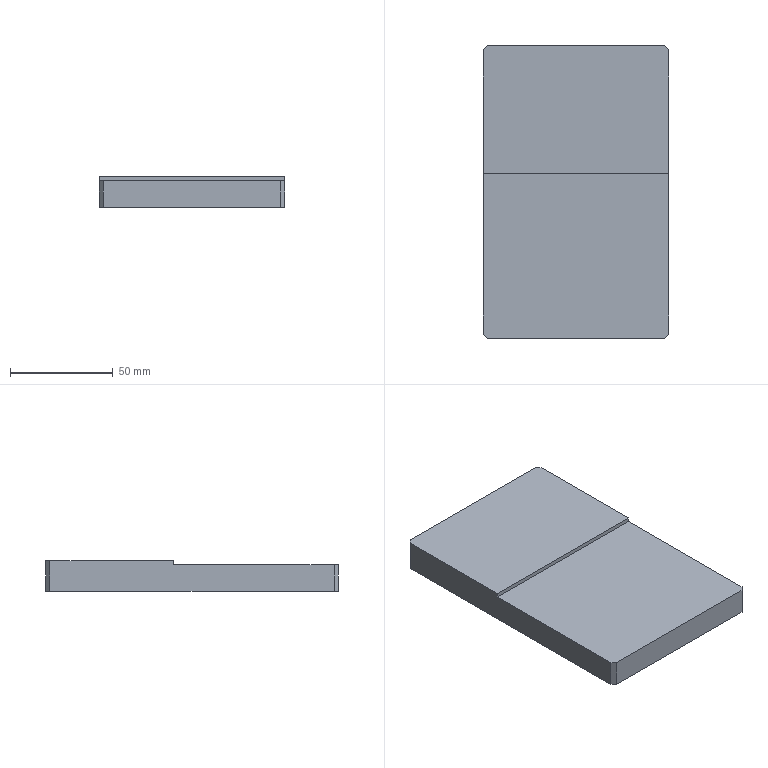Part | STEP file | 001-005-Shaft threading fixture adapter plate | 1 solid | 12 faces | box 90 x 142 x 15 mm | volume 177188 mm3 | plane 12
STEP:
#1=CARTESIAN_POINT('',(0.,0.,0.));
#2=DIRECTION('',(0.,0.,1.));
#3=DIRECTION('',(1.,0.,0.));
#4=AXIS2_PLACEMENT_3D('',#1,#2,#3);
#5=CARTESIAN_POINT('',(45.,9.,15.));
#6=VERTEX_POINT('',#5);
#7=CARTESIAN_POINT('',(45.,9.,13.));
#8=VERTEX_POINT('',#7);
#9=CARTESIAN_POINT('',(45.,9.,15.));
#10=DIRECTION('',(0.,0.,-1.));
#11=VECTOR('',#10,1.);
#12=LINE('',#9,#11);
#13=CARTESIAN_POINT('',(45.,-71.,15.));
#14=DIRECTION('',(-1.,0.,0.));
#15=DIRECTION('',(0.,-1.,0.));
#16=AXIS2_PLACEMENT_3D('',#13,#14,#15);
#17=PLANE('',#16);
#18=CARTESIAN_POINT('',(-80.,0.));
#19=DIRECTION('',(0.,-1.));
#20=VECTOR('',#19,1.);
#21=LINE('',#18,#20);
#22=(GEOMETRIC_REPRESENTATION_CONTEXT(2)PARAMETRIC_REPRESENTATION_CONTEXT()REPRESENTATION_CONTEXT('',''));
#23=DEFINITIONAL_REPRESENTATION('',(#21),#22);
#24=PCURVE('',#17,#23);
#25=CARTESIAN_POINT('',(45.,9.,15.));
#26=DIRECTION('',(0.,1.,0.));
#27=DIRECTION('',(0.,0.,1.));
#28=AXIS2_PLACEMENT_3D('',#25,#26,#27);
#29=PLANE('',#28);
#30=CARTESIAN_POINT('',(0.,0.));
#31=DIRECTION('',(-1.,0.));
#32=VECTOR('',#31,1.);
#33=LINE('',#30,#32);
#34=(GEOMETRIC_REPRESENTATION_CONTEXT(2)PARAMETRIC_REPRESENTATION_CONTEXT()REPRESENTATION_CONTEXT('',''));
#35=DEFINITIONAL_REPRESENTATION('',(#33),#34);
#36=PCURVE('',#29,#35);
#37=SURFACE_CURVE('',#12,(#24,#36),.PCURVE_S1.);
#38=EDGE_CURVE('',#6,#8,#37,.T.);
#39=ORIENTED_EDGE('',*,*,#38,.T.);
#40=CARTESIAN_POINT('',(45.,-69.,13.));
#41=VERTEX_POINT('',#40);
#42=CARTESIAN_POINT('',(45.,9.,13.));
#43=DIRECTION('',(0.,-1.,0.));
#44=VECTOR('',#43,1.);
#45=LINE('',#42,#44);
#46=CARTESIAN_POINT('',(-80.,-2.));
#47=DIRECTION('',(1.,0.));
#48=VECTOR('',#47,1.);
#49=LINE('',#46,#48);
#50=(GEOMETRIC_REPRESENTATION_CONTEXT(2)PARAMETRIC_REPRESENTATION_CONTEXT()REPRESENTATION_CONTEXT('',''));
#51=DEFINITIONAL_REPRESENTATION('',(#49),#50);
#52=PCURVE('',#17,#51);
#53=CARTESIAN_POINT('',(45.,9.,13.));
#54=DIRECTION('',(0.,0.,-1.));
#55=DIRECTION('',(0.,1.,0.));
#56=AXIS2_PLACEMENT_3D('',#53,#54,#55);
#57=PLANE('',#56);
#58=CARTESIAN_POINT('',(0.,0.));
#59=DIRECTION('',(-1.,0.));
#60=VECTOR('',#59,1.);
#61=LINE('',#58,#60);
#62=(GEOMETRIC_REPRESENTATION_CONTEXT(2)PARAMETRIC_REPRESENTATION_CONTEXT()REPRESENTATION_CONTEXT('',''));
#63=DEFINITIONAL_REPRESENTATION('',(#61),#62);
#64=PCURVE('',#57,#63);
#65=SURFACE_CURVE('',#45,(#52,#64),.PCURVE_S1.);
#66=EDGE_CURVE('',#8,#41,#65,.T.);
#67=ORIENTED_EDGE('',*,*,#66,.T.);
#68=CARTESIAN_POINT('',(45.,-69.,0.));
#69=VERTEX_POINT('',#68);
#70=CARTESIAN_POINT('',(45.,-69.,15.));
#71=DIRECTION('',(0.,0.,-1.));
#72=VECTOR('',#71,1.);
#73=LINE('',#70,#72);
#74=CARTESIAN_POINT('',(-2.,0.));
#75=DIRECTION('',(0.,-1.));
#76=VECTOR('',#75,1.);
#77=LINE('',#74,#76);
#78=(GEOMETRIC_REPRESENTATION_CONTEXT(2)PARAMETRIC_REPRESENTATION_CONTEXT()REPRESENTATION_CONTEXT('',''));
#79=DEFINITIONAL_REPRESENTATION('',(#77),#78);
#80=PCURVE('',#17,#79);
#81=CARTESIAN_POINT('',(45.,-69.,15.));
#82=DIRECTION('',(-0.7071,0.7071,0.));
#83=DIRECTION('',(0.,0.,-1.));
#84=AXIS2_PLACEMENT_3D('',#81,#82,#83);
#85=PLANE('',#84);
#86=CARTESIAN_POINT('',(0.,0.));
#87=DIRECTION('',(1.,0.));
#88=VECTOR('',#87,1.);
#89=LINE('',#86,#88);
#90=(GEOMETRIC_REPRESENTATION_CONTEXT(2)PARAMETRIC_REPRESENTATION_CONTEXT()REPRESENTATION_CONTEXT('',''));
#91=DEFINITIONAL_REPRESENTATION('',(#89),#90);
#92=PCURVE('',#85,#91);
#93=SURFACE_CURVE('',#73,(#80,#92),.PCURVE_S1.);
#94=EDGE_CURVE('',#41,#69,#93,.T.);
#95=ORIENTED_EDGE('',*,*,#94,.T.);
#96=CARTESIAN_POINT('',(45.,69.,0.));
#97=VERTEX_POINT('',#96);
#98=CARTESIAN_POINT('',(45.,-71.,0.));
#99=DIRECTION('',(0.,1.,0.));
#100=VECTOR('',#99,1.);
#101=LINE('',#98,#100);
#102=CARTESIAN_POINT('',(0.,-15.));
#103=DIRECTION('',(-1.,0.));
#104=VECTOR('',#103,1.);
#105=LINE('',#102,#104);
#106=(GEOMETRIC_REPRESENTATION_CONTEXT(2)PARAMETRIC_REPRESENTATION_CONTEXT()REPRESENTATION_CONTEXT('',''));
#107=DEFINITIONAL_REPRESENTATION('',(#105),#106);
#108=PCURVE('',#17,#107);
#109=CARTESIAN_POINT('',(0.,0.,0.));
#110=DIRECTION('',(0.,0.,-1.));
#111=DIRECTION('',(-1.,0.,0.));
#112=AXIS2_PLACEMENT_3D('',#109,#110,#111);
#113=PLANE('',#112);
#114=CARTESIAN_POINT('',(-45.,-71.));
#115=DIRECTION('',(0.,1.));
#116=VECTOR('',#115,1.);
#117=LINE('',#114,#116);
#118=(GEOMETRIC_REPRESENTATION_CONTEXT(2)PARAMETRIC_REPRESENTATION_CONTEXT()REPRESENTATION_CONTEXT('',''));
#119=DEFINITIONAL_REPRESENTATION('',(#117),#118);
#120=PCURVE('',#113,#119);
#121=SURFACE_CURVE('',#101,(#108,#120),.PCURVE_S1.);
#122=EDGE_CURVE('',#69,#97,#121,.T.);
#123=ORIENTED_EDGE('',*,*,#122,.T.);
#124=CARTESIAN_POINT('',(45.,69.,15.));
#125=VERTEX_POINT('',#124);
#126=CARTESIAN_POINT('',(45.,69.,15.));
#127=DIRECTION('',(0.,0.,1.));
#128=VECTOR('',#127,1.);
#129=LINE('',#126,#128);
#130=CARTESIAN_POINT('',(-140.,0.));
#131=DIRECTION('',(0.,1.));
#132=VECTOR('',#131,1.);
#133=LINE('',#130,#132);
#134=(GEOMETRIC_REPRESENTATION_CONTEXT(2)PARAMETRIC_REPRESENTATION_CONTEXT()REPRESENTATION_CONTEXT('',''));
#135=DEFINITIONAL_REPRESENTATION('',(#133),#134);
#136=PCURVE('',#17,#135);
#137=CARTESIAN_POINT('',(43.,71.,15.));
#138=DIRECTION('',(-0.7071,-0.7071,0.));
#139=DIRECTION('',(0.,0.,-1.));
#140=AXIS2_PLACEMENT_3D('',#137,#138,#139);
#141=PLANE('',#140);
#142=CARTESIAN_POINT('',(0.,2.828));
#143=DIRECTION('',(-1.,0.));
#144=VECTOR('',#143,1.);
#145=LINE('',#142,#144);
#146=(GEOMETRIC_REPRESENTATION_CONTEXT(2)PARAMETRIC_REPRESENTATION_CONTEXT()REPRESENTATION_CONTEXT('',''));
#147=DEFINITIONAL_REPRESENTATION('',(#145),#146);
#148=PCURVE('',#141,#147);
#149=SURFACE_CURVE('',#129,(#136,#148),.PCURVE_S1.);
#150=EDGE_CURVE('',#97,#125,#149,.T.);
#151=ORIENTED_EDGE('',*,*,#150,.T.);
#152=CARTESIAN_POINT('',(45.,-71.,15.));
#153=DIRECTION('',(0.,1.,0.));
#154=VECTOR('',#153,1.);
#155=LINE('',#152,#154);
#156=CARTESIAN_POINT('',(0.,0.));
#157=DIRECTION('',(-1.,0.));
#158=VECTOR('',#157,1.);
#159=LINE('',#156,#158);
#160=(GEOMETRIC_REPRESENTATION_CONTEXT(2)PARAMETRIC_REPRESENTATION_CONTEXT()REPRESENTATION_CONTEXT('',''));
#161=DEFINITIONAL_REPRESENTATION('',(#159),#160);
#162=PCURVE('',#17,#161);
#163=CARTESIAN_POINT('',(0.,0.,15.));
#164=DIRECTION('',(0.,0.,-1.));
#165=DIRECTION('',(-1.,0.,0.));
#166=AXIS2_PLACEMENT_3D('',#163,#164,#165);
#167=PLANE('',#166);
#168=CARTESIAN_POINT('',(-45.,-71.));
#169=DIRECTION('',(0.,1.));
#170=VECTOR('',#169,1.);
#171=LINE('',#168,#170);
#172=(GEOMETRIC_REPRESENTATION_CONTEXT(2)PARAMETRIC_REPRESENTATION_CONTEXT()REPRESENTATION_CONTEXT('',''));
#173=DEFINITIONAL_REPRESENTATION('',(#171),#172);
#174=PCURVE('',#167,#173);
#175=SURFACE_CURVE('',#155,(#162,#174),.PCURVE_S1.);
#176=EDGE_CURVE('',#6,#125,#175,.T.);
#177=ORIENTED_EDGE('',*,*,#176,.F.);
#178=EDGE_LOOP('',(#39,#67,#95,#123,#151,#177));
#179=FACE_BOUND('',#178,.T.);
#180=ADVANCED_FACE('',(#179),#17,.F.);
#181=CARTESIAN_POINT('',(43.,71.,0.));
#182=VERTEX_POINT('',#181);
#183=CARTESIAN_POINT('',(-43.,71.,0.));
#184=VERTEX_POINT('',#183);
#185=CARTESIAN_POINT('',(-45.,71.,0.));
#186=DIRECTION('',(-1.,0.,0.));
#187=VECTOR('',#186,1.);
#188=LINE('',#185,#187);
#189=CARTESIAN_POINT('',(-45.,71.,15.));
#190=DIRECTION('',(0.,-1.,0.));
#191=DIRECTION('',(0.,0.,-1.));
#192=AXIS2_PLACEMENT_3D('',#189,#190,#191);
#193=PLANE('',#192);
#194=CARTESIAN_POINT('',(15.,0.));
#195=DIRECTION('',(0.,-1.));
#196=VECTOR('',#195,1.);
#197=LINE('',#194,#196);
#198=(GEOMETRIC_REPRESENTATION_CONTEXT(2)PARAMETRIC_REPRESENTATION_CONTEXT()REPRESENTATION_CONTEXT('',''));
#199=DEFINITIONAL_REPRESENTATION('',(#197),#198);
#200=PCURVE('',#193,#199);
#201=CARTESIAN_POINT('',(45.,71.));
#202=DIRECTION('',(1.,0.));
#203=VECTOR('',#202,1.);
#204=LINE('',#201,#203);
#205=(GEOMETRIC_REPRESENTATION_CONTEXT(2)PARAMETRIC_REPRESENTATION_CONTEXT()REPRESENTATION_CONTEXT('',''));
#206=DEFINITIONAL_REPRESENTATION('',(#204),#205);
#207=PCURVE('',#113,#206);
#208=SURFACE_CURVE('',#188,(#200,#207),.PCURVE_S1.);
#209=EDGE_CURVE('',#182,#184,#208,.T.);
#210=ORIENTED_EDGE('',*,*,#209,.T.);
#211=CARTESIAN_POINT('',(-43.,71.,15.));
#212=VERTEX_POINT('',#211);
#213=CARTESIAN_POINT('',(-43.,71.,15.));
#214=DIRECTION('',(0.,0.,1.));
#215=VECTOR('',#214,1.);
#216=LINE('',#213,#215);
#217=CARTESIAN_POINT('',(0.,2.));
#218=DIRECTION('',(-1.,0.));
#219=VECTOR('',#218,1.);
#220=LINE('',#217,#219);
#221=(GEOMETRIC_REPRESENTATION_CONTEXT(2)PARAMETRIC_REPRESENTATION_CONTEXT()REPRESENTATION_CONTEXT('',''));
#222=DEFINITIONAL_REPRESENTATION('',(#220),#221);
#223=PCURVE('',#193,#222);
#224=CARTESIAN_POINT('',(-45.,69.,15.));
#225=DIRECTION('',(0.7071,-0.7071,0.));
#226=DIRECTION('',(0.,0.,-1.));
#227=AXIS2_PLACEMENT_3D('',#224,#225,#226);
#228=PLANE('',#227);
#229=CARTESIAN_POINT('',(0.,2.828));
#230=DIRECTION('',(-1.,0.));
#231=VECTOR('',#230,1.);
#232=LINE('',#229,#231);
#233=(GEOMETRIC_REPRESENTATION_CONTEXT(2)PARAMETRIC_REPRESENTATION_CONTEXT()REPRESENTATION_CONTEXT('',''));
#234=DEFINITIONAL_REPRESENTATION('',(#232),#233);
#235=PCURVE('',#228,#234);
#236=SURFACE_CURVE('',#216,(#223,#235),.PCURVE_S1.);
#237=EDGE_CURVE('',#184,#212,#236,.T.);
#238=ORIENTED_EDGE('',*,*,#237,.T.);
#239=CARTESIAN_POINT('',(43.,71.,15.));
#240=VERTEX_POINT('',#239);
#241=CARTESIAN_POINT('',(-45.,71.,15.));
#242=DIRECTION('',(-1.,0.,0.));
#243=VECTOR('',#242,1.);
#244=LINE('',#241,#243);
#245=CARTESIAN_POINT('',(0.,0.));
#246=DIRECTION('',(0.,-1.));
#247=VECTOR('',#246,1.);
#248=LINE('',#245,#247);
#249=(GEOMETRIC_REPRESENTATION_CONTEXT(2)PARAMETRIC_REPRESENTATION_CONTEXT()REPRESENTATION_CONTEXT('',''));
#250=DEFINITIONAL_REPRESENTATION('',(#248),#249);
#251=PCURVE('',#193,#250);
#252=CARTESIAN_POINT('',(45.,71.));
#253=DIRECTION('',(1.,0.));
#254=VECTOR('',#253,1.);
#255=LINE('',#252,#254);
#256=(GEOMETRIC_REPRESENTATION_CONTEXT(2)PARAMETRIC_REPRESENTATION_CONTEXT()REPRESENTATION_CONTEXT('',''));
#257=DEFINITIONAL_REPRESENTATION('',(#255),#256);
#258=PCURVE('',#167,#257);
#259=SURFACE_CURVE('',#244,(#251,#258),.PCURVE_S1.);
#260=EDGE_CURVE('',#240,#212,#259,.T.);
#261=ORIENTED_EDGE('',*,*,#260,.F.);
#262=CARTESIAN_POINT('',(43.,71.,15.));
#263=DIRECTION('',(0.,0.,-1.));
#264=VECTOR('',#263,1.);
#265=LINE('',#262,#264);
#266=CARTESIAN_POINT('',(0.,88.));
#267=DIRECTION('',(1.,0.));
#268=VECTOR('',#267,1.);
#269=LINE('',#266,#268);
#270=(GEOMETRIC_REPRESENTATION_CONTEXT(2)PARAMETRIC_REPRESENTATION_CONTEXT()REPRESENTATION_CONTEXT('',''));
#271=DEFINITIONAL_REPRESENTATION('',(#269),#270);
#272=PCURVE('',#193,#271);
#273=CARTESIAN_POINT('',(0.,0.));
#274=DIRECTION('',(1.,0.));
#275=VECTOR('',#274,1.);
#276=LINE('',#273,#275);
#277=(GEOMETRIC_REPRESENTATION_CONTEXT(2)PARAMETRIC_REPRESENTATION_CONTEXT()REPRESENTATION_CONTEXT('',''));
#278=DEFINITIONAL_REPRESENTATION('',(#276),#277);
#279=PCURVE('',#141,#278);
#280=SURFACE_CURVE('',#265,(#272,#279),.PCURVE_S1.);
#281=EDGE_CURVE('',#240,#182,#280,.T.);
#282=ORIENTED_EDGE('',*,*,#281,.T.);
#283=EDGE_LOOP('',(#210,#238,#261,#282));
#284=FACE_BOUND('',#283,.T.);
#285=ADVANCED_FACE('',(#284),#193,.F.);
#286=CARTESIAN_POINT('',(-45.,-69.,0.));
#287=VERTEX_POINT('',#286);
#288=CARTESIAN_POINT('',(-45.,-69.,13.));
#289=VERTEX_POINT('',#288);
#290=CARTESIAN_POINT('',(-45.,-69.,15.));
#291=DIRECTION('',(0.,0.,1.));
#292=VECTOR('',#291,1.);
#293=LINE('',#290,#292);
#294=CARTESIAN_POINT('',(-45.,-71.,15.));
#295=DIRECTION('',(1.,0.,0.));
#296=DIRECTION('',(0.,0.,-1.));
#297=AXIS2_PLACEMENT_3D('',#294,#295,#296);
#298=PLANE('',#297);
#299=CARTESIAN_POINT('',(0.,2.));
#300=DIRECTION('',(-1.,0.));
#301=VECTOR('',#300,1.);
#302=LINE('',#299,#301);
#303=(GEOMETRIC_REPRESENTATION_CONTEXT(2)PARAMETRIC_REPRESENTATION_CONTEXT()REPRESENTATION_CONTEXT('',''));
#304=DEFINITIONAL_REPRESENTATION('',(#302),#303);
#305=PCURVE('',#298,#304);
#306=CARTESIAN_POINT('',(-43.,-71.,15.));
#307=DIRECTION('',(0.7071,0.7071,0.));
#308=DIRECTION('',(0.,0.,-1.));
#309=AXIS2_PLACEMENT_3D('',#306,#307,#308);
#310=PLANE('',#309);
#311=CARTESIAN_POINT('',(0.,2.828));
#312=DIRECTION('',(-1.,0.));
#313=VECTOR('',#312,1.);
#314=LINE('',#311,#313);
#315=(GEOMETRIC_REPRESENTATION_CONTEXT(2)PARAMETRIC_REPRESENTATION_CONTEXT()REPRESENTATION_CONTEXT('',''));
#316=DEFINITIONAL_REPRESENTATION('',(#314),#315);
#317=PCURVE('',#310,#316);
#318=SURFACE_CURVE('',#293,(#305,#317),.PCURVE_S1.);
#319=EDGE_CURVE('',#287,#289,#318,.T.);
#320=ORIENTED_EDGE('',*,*,#319,.T.);
#321=CARTESIAN_POINT('',(-45.,9.,13.));
#322=VERTEX_POINT('',#321);
#323=CARTESIAN_POINT('',(-45.,9.,13.));
#324=DIRECTION('',(0.,-1.,0.));
#325=VECTOR('',#324,1.);
#326=LINE('',#323,#325);
#327=CARTESIAN_POINT('',(2.,80.));
#328=DIRECTION('',(0.,-1.));
#329=VECTOR('',#328,1.);
#330=LINE('',#327,#329);
#331=(GEOMETRIC_REPRESENTATION_CONTEXT(2)PARAMETRIC_REPRESENTATION_CONTEXT()REPRESENTATION_CONTEXT('',''));
#332=DEFINITIONAL_REPRESENTATION('',(#330),#331);
#333=PCURVE('',#298,#332);
#334=CARTESIAN_POINT('',(0.,-90.));
#335=DIRECTION('',(-1.,0.));
#336=VECTOR('',#335,1.);
#337=LINE('',#334,#336);
#338=(GEOMETRIC_REPRESENTATION_CONTEXT(2)PARAMETRIC_REPRESENTATION_CONTEXT()REPRESENTATION_CONTEXT('',''));
#339=DEFINITIONAL_REPRESENTATION('',(#337),#338);
#340=PCURVE('',#57,#339);
#341=SURFACE_CURVE('',#326,(#333,#340),.PCURVE_S1.);
#342=EDGE_CURVE('',#322,#289,#341,.T.);
#343=ORIENTED_EDGE('',*,*,#342,.F.);
#344=CARTESIAN_POINT('',(-45.,9.,15.));
#345=VERTEX_POINT('',#344);
#346=CARTESIAN_POINT('',(-45.,9.,15.));
#347=DIRECTION('',(0.,0.,-1.));
#348=VECTOR('',#347,1.);
#349=LINE('',#346,#348);
#350=CARTESIAN_POINT('',(0.,80.));
#351=DIRECTION('',(1.,0.));
#352=VECTOR('',#351,1.);
#353=LINE('',#350,#352);
#354=(GEOMETRIC_REPRESENTATION_CONTEXT(2)PARAMETRIC_REPRESENTATION_CONTEXT()REPRESENTATION_CONTEXT('',''));
#355=DEFINITIONAL_REPRESENTATION('',(#353),#354);
#356=PCURVE('',#298,#355);
#357=CARTESIAN_POINT('',(0.,-90.));
#358=DIRECTION('',(-1.,0.));
#359=VECTOR('',#358,1.);
#360=LINE('',#357,#359);
#361=(GEOMETRIC_REPRESENTATION_CONTEXT(2)PARAMETRIC_REPRESENTATION_CONTEXT()REPRESENTATION_CONTEXT('',''));
#362=DEFINITIONAL_REPRESENTATION('',(#360),#361);
#363=PCURVE('',#29,#362);
#364=SURFACE_CURVE('',#349,(#356,#363),.PCURVE_S1.);
#365=EDGE_CURVE('',#345,#322,#364,.T.);
#366=ORIENTED_EDGE('',*,*,#365,.F.);
#367=CARTESIAN_POINT('',(-45.,69.,15.));
#368=VERTEX_POINT('',#367);
#369=CARTESIAN_POINT('',(-45.,-71.,15.));
#370=DIRECTION('',(0.,-1.,0.));
#371=VECTOR('',#370,1.);
#372=LINE('',#369,#371);
#373=CARTESIAN_POINT('',(0.,0.));
#374=DIRECTION('',(0.,-1.));
#375=VECTOR('',#374,1.);
#376=LINE('',#373,#375);
#377=(GEOMETRIC_REPRESENTATION_CONTEXT(2)PARAMETRIC_REPRESENTATION_CONTEXT()REPRESENTATION_CONTEXT('',''));
#378=DEFINITIONAL_REPRESENTATION('',(#376),#377);
#379=PCURVE('',#298,#378);
#380=CARTESIAN_POINT('',(45.,-71.));
#381=DIRECTION('',(0.,-1.));
#382=VECTOR('',#381,1.);
#383=LINE('',#380,#382);
#384=(GEOMETRIC_REPRESENTATION_CONTEXT(2)PARAMETRIC_REPRESENTATION_CONTEXT()REPRESENTATION_CONTEXT('',''));
#385=DEFINITIONAL_REPRESENTATION('',(#383),#384);
#386=PCURVE('',#167,#385);
#387=SURFACE_CURVE('',#372,(#379,#386),.PCURVE_S1.);
#388=EDGE_CURVE('',#368,#345,#387,.T.);
#389=ORIENTED_EDGE('',*,*,#388,.F.);
#390=CARTESIAN_POINT('',(-45.,69.,0.));
#391=VERTEX_POINT('',#390);
#392=CARTESIAN_POINT('',(-45.,69.,15.));
#393=DIRECTION('',(0.,0.,-1.));
#394=VECTOR('',#393,1.);
#395=LINE('',#392,#394);
#396=CARTESIAN_POINT('',(0.,140.));
#397=DIRECTION('',(1.,0.));
#398=VECTOR('',#397,1.);
#399=LINE('',#396,#398);
#400=(GEOMETRIC_REPRESENTATION_CONTEXT(2)PARAMETRIC_REPRESENTATION_CONTEXT()REPRESENTATION_CONTEXT('',''));
#401=DEFINITIONAL_REPRESENTATION('',(#399),#400);
#402=PCURVE('',#298,#401);
#403=CARTESIAN_POINT('',(0.,0.));
#404=DIRECTION('',(1.,0.));
#405=VECTOR('',#404,1.);
#406=LINE('',#403,#405);
#407=(GEOMETRIC_REPRESENTATION_CONTEXT(2)PARAMETRIC_REPRESENTATION_CONTEXT()REPRESENTATION_CONTEXT('',''));
#408=DEFINITIONAL_REPRESENTATION('',(#406),#407);
#409=PCURVE('',#228,#408);
#410=SURFACE_CURVE('',#395,(#402,#409),.PCURVE_S1.);
#411=EDGE_CURVE('',#368,#391,#410,.T.);
#412=ORIENTED_EDGE('',*,*,#411,.T.);
#413=CARTESIAN_POINT('',(-45.,-71.,0.));
#414=DIRECTION('',(0.,-1.,0.));
#415=VECTOR('',#414,1.);
#416=LINE('',#413,#415);
#417=CARTESIAN_POINT('',(15.,0.));
#418=DIRECTION('',(0.,-1.));
#419=VECTOR('',#418,1.);
#420=LINE('',#417,#419);
#421=(GEOMETRIC_REPRESENTATION_CONTEXT(2)PARAMETRIC_REPRESENTATION_CONTEXT()REPRESENTATION_CONTEXT('',''));
#422=DEFINITIONAL_REPRESENTATION('',(#420),#421);
#423=PCURVE('',#298,#422);
#424=CARTESIAN_POINT('',(45.,-71.));
#425=DIRECTION('',(0.,-1.));
#426=VECTOR('',#425,1.);
#427=LINE('',#424,#426);
#428=(GEOMETRIC_REPRESENTATION_CONTEXT(2)PARAMETRIC_REPRESENTATION_CONTEXT()REPRESENTATION_CONTEXT('',''));
#429=DEFINITIONAL_REPRESENTATION('',(#427),#428);
#430=PCURVE('',#113,#429);
#431=SURFACE_CURVE('',#416,(#423,#430),.PCURVE_S1.);
#432=EDGE_CURVE('',#391,#287,#431,.T.);
#433=ORIENTED_EDGE('',*,*,#432,.T.);
#434=EDGE_LOOP('',(#320,#343,#366,#389,#412,#433));
#435=FACE_BOUND('',#434,.T.);
#436=ADVANCED_FACE('',(#435),#298,.F.);
#437=CARTESIAN_POINT('',(43.,-71.,0.));
#438=VERTEX_POINT('',#437);
#439=CARTESIAN_POINT('',(43.,-71.,13.));
#440=VERTEX_POINT('',#439);
#441=CARTESIAN_POINT('',(43.,-71.,15.));
#442=DIRECTION('',(0.,0.,1.));
#443=VECTOR('',#442,1.);
#444=LINE('',#441,#443);
#445=CARTESIAN_POINT('',(-45.,-71.,15.));
#446=DIRECTION('',(0.,1.,0.));
#447=DIRECTION('',(0.,0.,1.));
#448=AXIS2_PLACEMENT_3D('',#445,#446,#447);
#449=PLANE('',#448);
#450=CARTESIAN_POINT('',(0.,88.));
#451=DIRECTION('',(1.,0.));
#452=VECTOR('',#451,1.);
#453=LINE('',#450,#452);
#454=(GEOMETRIC_REPRESENTATION_CONTEXT(2)PARAMETRIC_REPRESENTATION_CONTEXT()REPRESENTATION_CONTEXT('',''));
#455=DEFINITIONAL_REPRESENTATION('',(#453),#454);
#456=PCURVE('',#449,#455);
#457=CARTESIAN_POINT('',(0.,2.828));
#458=DIRECTION('',(-1.,0.));
#459=VECTOR('',#458,1.);
#460=LINE('',#457,#459);
#461=(GEOMETRIC_REPRESENTATION_CONTEXT(2)PARAMETRIC_REPRESENTATION_CONTEXT()REPRESENTATION_CONTEXT('',''));
#462=DEFINITIONAL_REPRESENTATION('',(#460),#461);
#463=PCURVE('',#85,#462);
#464=SURFACE_CURVE('',#444,(#456,#463),.PCURVE_S1.);
#465=EDGE_CURVE('',#438,#440,#464,.T.);
#466=ORIENTED_EDGE('',*,*,#465,.T.);
#467=CARTESIAN_POINT('',(-43.,-71.,13.));
#468=VERTEX_POINT('',#467);
#469=CARTESIAN_POINT('',(45.,-71.,13.));
#470=DIRECTION('',(-1.,0.,0.));
#471=VECTOR('',#470,1.);
#472=LINE('',#469,#471);
#473=CARTESIAN_POINT('',(-2.,90.));
#474=DIRECTION('',(0.,-1.));
#475=VECTOR('',#474,1.);
#476=LINE('',#473,#475);
#477=(GEOMETRIC_REPRESENTATION_CONTEXT(2)PARAMETRIC_REPRESENTATION_CONTEXT()REPRESENTATION_CONTEXT('',''));
#478=DEFINITIONAL_REPRESENTATION('',(#476),#477);
#479=PCURVE('',#449,#478);
#480=CARTESIAN_POINT('',(-80.,0.));
#481=DIRECTION('',(0.,-1.));
#482=VECTOR('',#481,1.);
#483=LINE('',#480,#482);
#484=(GEOMETRIC_REPRESENTATION_CONTEXT(2)PARAMETRIC_REPRESENTATION_CONTEXT()REPRESENTATION_CONTEXT('',''));
#485=DEFINITIONAL_REPRESENTATION('',(#483),#484);
#486=PCURVE('',#57,#485);
#487=SURFACE_CURVE('',#472,(#479,#486),.PCURVE_S1.);
#488=EDGE_CURVE('',#440,#468,#487,.T.);
#489=ORIENTED_EDGE('',*,*,#488,.T.);
#490=CARTESIAN_POINT('',(-43.,-71.,0.));
#491=VERTEX_POINT('',#490);
#492=CARTESIAN_POINT('',(-43.,-71.,15.));
#493=DIRECTION('',(0.,0.,-1.));
#494=VECTOR('',#493,1.);
#495=LINE('',#492,#494);
#496=CARTESIAN_POINT('',(0.,2.));
#497=DIRECTION('',(-1.,0.));
#498=VECTOR('',#497,1.);
#499=LINE('',#496,#498);
#500=(GEOMETRIC_REPRESENTATION_CONTEXT(2)PARAMETRIC_REPRESENTATION_CONTEXT()REPRESENTATION_CONTEXT('',''));
#501=DEFINITIONAL_REPRESENTATION('',(#499),#500);
#502=PCURVE('',#449,#501);
#503=CARTESIAN_POINT('',(0.,0.));
#504=DIRECTION('',(1.,0.));
#505=VECTOR('',#504,1.);
#506=LINE('',#503,#505);
#507=(GEOMETRIC_REPRESENTATION_CONTEXT(2)PARAMETRIC_REPRESENTATION_CONTEXT()REPRESENTATION_CONTEXT('',''));
#508=DEFINITIONAL_REPRESENTATION('',(#506),#507);
#509=PCURVE('',#310,#508);
#510=SURFACE_CURVE('',#495,(#502,#509),.PCURVE_S1.);
#511=EDGE_CURVE('',#468,#491,#510,.T.);
#512=ORIENTED_EDGE('',*,*,#511,.T.);
#513=CARTESIAN_POINT('',(-45.,-71.,0.));
#514=DIRECTION('',(1.,0.,0.));
#515=VECTOR('',#514,1.);
#516=LINE('',#513,#515);
#517=CARTESIAN_POINT('',(-15.,0.));
#518=DIRECTION('',(0.,1.));
#519=VECTOR('',#518,1.);
#520=LINE('',#517,#519);
#521=(GEOMETRIC_REPRESENTATION_CONTEXT(2)PARAMETRIC_REPRESENTATION_CONTEXT()REPRESENTATION_CONTEXT('',''));
#522=DEFINITIONAL_REPRESENTATION('',(#520),#521);
#523=PCURVE('',#449,#522);
#524=CARTESIAN_POINT('',(45.,-71.));
#525=DIRECTION('',(-1.,0.));
#526=VECTOR('',#525,1.);
#527=LINE('',#524,#526);
#528=(GEOMETRIC_REPRESENTATION_CONTEXT(2)PARAMETRIC_REPRESENTATION_CONTEXT()REPRESENTATION_CONTEXT('',''));
#529=DEFINITIONAL_REPRESENTATION('',(#527),#528);
#530=PCURVE('',#113,#529);
#531=SURFACE_CURVE('',#516,(#523,#530),.PCURVE_S1.);
#532=EDGE_CURVE('',#491,#438,#531,.T.);
#533=ORIENTED_EDGE('',*,*,#532,.T.);
#534=EDGE_LOOP('',(#466,#489,#512,#533));
#535=FACE_BOUND('',#534,.T.);
#536=ADVANCED_FACE('',(#535),#449,.F.);
#537=ORIENTED_EDGE('',*,*,#388,.T.);
#538=CARTESIAN_POINT('',(45.,9.,15.));
#539=DIRECTION('',(-1.,0.,0.));
#540=VECTOR('',#539,1.);
#541=LINE('',#538,#540);
#542=CARTESIAN_POINT('',(-45.,9.));
#543=DIRECTION('',(1.,0.));
#544=VECTOR('',#543,1.);
#545=LINE('',#542,#544);
#546=(GEOMETRIC_REPRESENTATION_CONTEXT(2)PARAMETRIC_REPRESENTATION_CONTEXT()REPRESENTATION_CONTEXT('',''));
#547=DEFINITIONAL_REPRESENTATION('',(#545),#546);
#548=PCURVE('',#167,#547);
#549=CARTESIAN_POINT('',(0.,0.));
#550=DIRECTION('',(0.,-1.));
#551=VECTOR('',#550,1.);
#552=LINE('',#549,#551);
#553=(GEOMETRIC_REPRESENTATION_CONTEXT(2)PARAMETRIC_REPRESENTATION_CONTEXT()REPRESENTATION_CONTEXT('',''));
#554=DEFINITIONAL_REPRESENTATION('',(#552),#553);
#555=PCURVE('',#29,#554);
#556=SURFACE_CURVE('',#541,(#548,#555),.PCURVE_S1.);
#557=EDGE_CURVE('',#6,#345,#556,.T.);
#558=ORIENTED_EDGE('',*,*,#557,.F.);
#559=ORIENTED_EDGE('',*,*,#176,.T.);
#560=CARTESIAN_POINT('',(43.,71.,15.));
#561=DIRECTION('',(-0.7071,0.7071,0.));
#562=VECTOR('',#561,1.);
#563=LINE('',#560,#562);
#564=CARTESIAN_POINT('',(-43.,71.));
#565=DIRECTION('',(0.7071,0.7071));
#566=VECTOR('',#565,1.);
#567=LINE('',#564,#566);
#568=(GEOMETRIC_REPRESENTATION_CONTEXT(2)PARAMETRIC_REPRESENTATION_CONTEXT()REPRESENTATION_CONTEXT('',''));
#569=DEFINITIONAL_REPRESENTATION('',(#567),#568);
#570=PCURVE('',#167,#569);
#571=CARTESIAN_POINT('',(0.,0.));
#572=DIRECTION('',(0.,-1.));
#573=VECTOR('',#572,1.);
#574=LINE('',#571,#573);
#575=(GEOMETRIC_REPRESENTATION_CONTEXT(2)PARAMETRIC_REPRESENTATION_CONTEXT()REPRESENTATION_CONTEXT('',''));
#576=DEFINITIONAL_REPRESENTATION('',(#574),#575);
#577=PCURVE('',#141,#576);
#578=SURFACE_CURVE('',#563,(#570,#577),.PCURVE_S1.);
#579=EDGE_CURVE('',#125,#240,#578,.T.);
#580=ORIENTED_EDGE('',*,*,#579,.T.);
#581=ORIENTED_EDGE('',*,*,#260,.T.);
#582=CARTESIAN_POINT('',(-45.,69.,15.));
#583=DIRECTION('',(-0.7071,-0.7071,0.));
#584=VECTOR('',#583,1.);
#585=LINE('',#582,#584);
#586=CARTESIAN_POINT('',(45.,69.));
#587=DIRECTION('',(0.7071,-0.7071));
#588=VECTOR('',#587,1.);
#589=LINE('',#586,#588);
#590=(GEOMETRIC_REPRESENTATION_CONTEXT(2)PARAMETRIC_REPRESENTATION_CONTEXT()REPRESENTATION_CONTEXT('',''));
#591=DEFINITIONAL_REPRESENTATION('',(#589),#590);
#592=PCURVE('',#167,#591);
#593=CARTESIAN_POINT('',(0.,0.));
#594=DIRECTION('',(0.,-1.));
#595=VECTOR('',#594,1.);
#596=LINE('',#593,#595);
#597=(GEOMETRIC_REPRESENTATION_CONTEXT(2)PARAMETRIC_REPRESENTATION_CONTEXT()REPRESENTATION_CONTEXT('',''));
#598=DEFINITIONAL_REPRESENTATION('',(#596),#597);
#599=PCURVE('',#228,#598);
#600=SURFACE_CURVE('',#585,(#592,#599),.PCURVE_S1.);
#601=EDGE_CURVE('',#212,#368,#600,.T.);
#602=ORIENTED_EDGE('',*,*,#601,.T.);
#603=EDGE_LOOP('',(#537,#558,#559,#580,#581,#602));
#604=FACE_BOUND('',#603,.T.);
#605=ADVANCED_FACE('',(#604),#167,.F.);
#606=ORIENTED_EDGE('',*,*,#122,.F.);
#607=CARTESIAN_POINT('',(57.,-57.,0.));
#608=DIRECTION('',(-0.7071,-0.7071,0.));
#609=VECTOR('',#608,1.);
#610=LINE('',#607,#609);
#611=CARTESIAN_POINT('',(-57.,-57.));
#612=DIRECTION('',(0.7071,-0.7071));
#613=VECTOR('',#612,1.);
#614=LINE('',#611,#613);
#615=(GEOMETRIC_REPRESENTATION_CONTEXT(2)PARAMETRIC_REPRESENTATION_CONTEXT()REPRESENTATION_CONTEXT('',''));
#616=DEFINITIONAL_REPRESENTATION('',(#614),#615);
#617=PCURVE('',#113,#616);
#618=CARTESIAN_POINT('',(15.,-16.971));
#619=DIRECTION('',(0.,1.));
#620=VECTOR('',#619,1.);
#621=LINE('',#618,#620);
#622=(GEOMETRIC_REPRESENTATION_CONTEXT(2)PARAMETRIC_REPRESENTATION_CONTEXT()REPRESENTATION_CONTEXT('',''));
#623=DEFINITIONAL_REPRESENTATION('',(#621),#622);
#624=PCURVE('',#85,#623);
#625=SURFACE_CURVE('',#610,(#617,#624),.PCURVE_S1.);
#626=EDGE_CURVE('',#69,#438,#625,.T.);
#627=ORIENTED_EDGE('',*,*,#626,.T.);
#628=ORIENTED_EDGE('',*,*,#532,.F.);
#629=CARTESIAN_POINT('',(-57.,-57.,0.));
#630=DIRECTION('',(-0.7071,0.7071,0.));
#631=VECTOR('',#630,1.);
#632=LINE('',#629,#631);
#633=CARTESIAN_POINT('',(57.,-57.));
#634=DIRECTION('',(0.7071,0.7071));
#635=VECTOR('',#634,1.);
#636=LINE('',#633,#635);
#637=(GEOMETRIC_REPRESENTATION_CONTEXT(2)PARAMETRIC_REPRESENTATION_CONTEXT()REPRESENTATION_CONTEXT('',''));
#638=DEFINITIONAL_REPRESENTATION('',(#636),#637);
#639=PCURVE('',#113,#638);
#640=CARTESIAN_POINT('',(15.,19.799));
#641=DIRECTION('',(0.,1.));
#642=VECTOR('',#641,1.);
#643=LINE('',#640,#642);
#644=(GEOMETRIC_REPRESENTATION_CONTEXT(2)PARAMETRIC_REPRESENTATION_CONTEXT()REPRESENTATION_CONTEXT('',''));
#645=DEFINITIONAL_REPRESENTATION('',(#643),#644);
#646=PCURVE('',#310,#645);
#647=SURFACE_CURVE('',#632,(#639,#646),.PCURVE_S1.);
#648=EDGE_CURVE('',#491,#287,#647,.T.);
#649=ORIENTED_EDGE('',*,*,#648,.T.);
#650=ORIENTED_EDGE('',*,*,#432,.F.);
#651=CARTESIAN_POINT('',(-57.,57.,0.));
#652=DIRECTION('',(0.7071,0.7071,0.));
#653=VECTOR('',#652,1.);
#654=LINE('',#651,#653);
#655=CARTESIAN_POINT('',(57.,57.));
#656=DIRECTION('',(-0.7071,0.7071));
#657=VECTOR('',#656,1.);
#658=LINE('',#655,#657);
#659=(GEOMETRIC_REPRESENTATION_CONTEXT(2)PARAMETRIC_REPRESENTATION_CONTEXT()REPRESENTATION_CONTEXT('',''));
#660=DEFINITIONAL_REPRESENTATION('',(#658),#659);
#661=PCURVE('',#113,#660);
#662=CARTESIAN_POINT('',(15.,-16.971));
#663=DIRECTION('',(0.,1.));
#664=VECTOR('',#663,1.);
#665=LINE('',#662,#664);
#666=(GEOMETRIC_REPRESENTATION_CONTEXT(2)PARAMETRIC_REPRESENTATION_CONTEXT()REPRESENTATION_CONTEXT('',''));
#667=DEFINITIONAL_REPRESENTATION('',(#665),#666);
#668=PCURVE('',#228,#667);
#669=SURFACE_CURVE('',#654,(#661,#668),.PCURVE_S1.);
#670=EDGE_CURVE('',#391,#184,#669,.T.);
#671=ORIENTED_EDGE('',*,*,#670,.T.);
#672=ORIENTED_EDGE('',*,*,#209,.F.);
#673=CARTESIAN_POINT('',(57.,57.,0.));
#674=DIRECTION('',(0.7071,-0.7071,0.));
#675=VECTOR('',#674,1.);
#676=LINE('',#673,#675);
#677=CARTESIAN_POINT('',(-57.,57.));
#678=DIRECTION('',(-0.7071,-0.7071));
#679=VECTOR('',#678,1.);
#680=LINE('',#677,#679);
#681=(GEOMETRIC_REPRESENTATION_CONTEXT(2)PARAMETRIC_REPRESENTATION_CONTEXT()REPRESENTATION_CONTEXT('',''));
#682=DEFINITIONAL_REPRESENTATION('',(#680),#681);
#683=PCURVE('',#113,#682);
#684=CARTESIAN_POINT('',(15.,19.799));
#685=DIRECTION('',(0.,1.));
#686=VECTOR('',#685,1.);
#687=LINE('',#684,#686);
#688=(GEOMETRIC_REPRESENTATION_CONTEXT(2)PARAMETRIC_REPRESENTATION_CONTEXT()REPRESENTATION_CONTEXT('',''));
#689=DEFINITIONAL_REPRESENTATION('',(#687),#688);
#690=PCURVE('',#141,#689);
#691=SURFACE_CURVE('',#676,(#683,#690),.PCURVE_S1.);
#692=EDGE_CURVE('',#182,#97,#691,.T.);
#693=ORIENTED_EDGE('',*,*,#692,.T.);
#694=EDGE_LOOP('',(#606,#627,#628,#649,#650,#671,#672,#693));
#695=FACE_BOUND('',#694,.T.);
#696=ADVANCED_FACE('',(#695),#113,.T.);
#697=CARTESIAN_POINT('',(45.,-69.,13.));
#698=DIRECTION('',(0.7071,0.7071,0.));
#699=VECTOR('',#698,1.);
#700=LINE('',#697,#699);
#701=CARTESIAN_POINT('',(2.,0.));
#702=DIRECTION('',(0.,-1.));
#703=VECTOR('',#702,1.);
#704=LINE('',#701,#703);
#705=(GEOMETRIC_REPRESENTATION_CONTEXT(2)PARAMETRIC_REPRESENTATION_CONTEXT()REPRESENTATION_CONTEXT('',''));
#706=DEFINITIONAL_REPRESENTATION('',(#704),#705);
#707=PCURVE('',#85,#706);
#708=CARTESIAN_POINT('',(-78.,0.));
#709=DIRECTION('',(0.7071,0.7071));
#710=VECTOR('',#709,1.);
#711=LINE('',#708,#710);
#712=(GEOMETRIC_REPRESENTATION_CONTEXT(2)PARAMETRIC_REPRESENTATION_CONTEXT()REPRESENTATION_CONTEXT('',''));
#713=DEFINITIONAL_REPRESENTATION('',(#711),#712);
#714=PCURVE('',#57,#713);
#715=SURFACE_CURVE('',#700,(#707,#714),.PCURVE_S1.);
#716=EDGE_CURVE('',#440,#41,#715,.T.);
#717=ORIENTED_EDGE('',*,*,#716,.F.);
#718=ORIENTED_EDGE('',*,*,#465,.F.);
#719=ORIENTED_EDGE('',*,*,#626,.F.);
#720=ORIENTED_EDGE('',*,*,#94,.F.);
#721=EDGE_LOOP('',(#717,#718,#719,#720));
#722=FACE_BOUND('',#721,.T.);
#723=ADVANCED_FACE('',(#722),#85,.F.);
#724=CARTESIAN_POINT('',(-43.,-71.,13.));
#725=DIRECTION('',(0.7071,-0.7071,0.));
#726=VECTOR('',#725,1.);
#727=LINE('',#724,#726);
#728=CARTESIAN_POINT('',(2.,0.));
#729=DIRECTION('',(0.,-1.));
#730=VECTOR('',#729,1.);
#731=LINE('',#728,#730);
#732=(GEOMETRIC_REPRESENTATION_CONTEXT(2)PARAMETRIC_REPRESENTATION_CONTEXT()REPRESENTATION_CONTEXT('',''));
#733=DEFINITIONAL_REPRESENTATION('',(#731),#732);
#734=PCURVE('',#310,#733);
#735=CARTESIAN_POINT('',(-80.,-88.));
#736=DIRECTION('',(-0.7071,0.7071));
#737=VECTOR('',#736,1.);
#738=LINE('',#735,#737);
#739=(GEOMETRIC_REPRESENTATION_CONTEXT(2)PARAMETRIC_REPRESENTATION_CONTEXT()REPRESENTATION_CONTEXT('',''));
#740=DEFINITIONAL_REPRESENTATION('',(#738),#739);
#741=PCURVE('',#57,#740);
#742=SURFACE_CURVE('',#727,(#734,#741),.PCURVE_S1.);
#743=EDGE_CURVE('',#289,#468,#742,.T.);
#744=ORIENTED_EDGE('',*,*,#743,.F.);
#745=ORIENTED_EDGE('',*,*,#319,.F.);
#746=ORIENTED_EDGE('',*,*,#648,.F.);
#747=ORIENTED_EDGE('',*,*,#511,.F.);
#748=EDGE_LOOP('',(#744,#745,#746,#747));
#749=FACE_BOUND('',#748,.T.);
#750=ADVANCED_FACE('',(#749),#310,.F.);
#751=ORIENTED_EDGE('',*,*,#601,.F.);
#752=ORIENTED_EDGE('',*,*,#237,.F.);
#753=ORIENTED_EDGE('',*,*,#670,.F.);
#754=ORIENTED_EDGE('',*,*,#411,.F.);
#755=EDGE_LOOP('',(#751,#752,#753,#754));
#756=FACE_BOUND('',#755,.T.);
#757=ADVANCED_FACE('',(#756),#228,.F.);
#758=ORIENTED_EDGE('',*,*,#579,.F.);
#759=ORIENTED_EDGE('',*,*,#150,.F.);
#760=ORIENTED_EDGE('',*,*,#692,.F.);
#761=ORIENTED_EDGE('',*,*,#281,.F.);
#762=EDGE_LOOP('',(#758,#759,#760,#761));
#763=FACE_BOUND('',#762,.T.);
#764=ADVANCED_FACE('',(#763),#141,.F.);
#765=ORIENTED_EDGE('',*,*,#716,.T.);
#766=ORIENTED_EDGE('',*,*,#66,.F.);
#767=CARTESIAN_POINT('',(45.,9.,13.));
#768=DIRECTION('',(-1.,0.,0.));
#769=VECTOR('',#768,1.);
#770=LINE('',#767,#769);
#771=CARTESIAN_POINT('',(0.,0.));
#772=DIRECTION('',(0.,-1.));
#773=VECTOR('',#772,1.);
#774=LINE('',#771,#773);
#775=(GEOMETRIC_REPRESENTATION_CONTEXT(2)PARAMETRIC_REPRESENTATION_CONTEXT()REPRESENTATION_CONTEXT('',''));
#776=DEFINITIONAL_REPRESENTATION('',(#774),#775);
#777=PCURVE('',#57,#776);
#778=CARTESIAN_POINT('',(-2.,0.));
#779=DIRECTION('',(0.,-1.));
#780=VECTOR('',#779,1.);
#781=LINE('',#778,#780);
#782=(GEOMETRIC_REPRESENTATION_CONTEXT(2)PARAMETRIC_REPRESENTATION_CONTEXT()REPRESENTATION_CONTEXT('',''));
#783=DEFINITIONAL_REPRESENTATION('',(#781),#782);
#784=PCURVE('',#29,#783);
#785=SURFACE_CURVE('',#770,(#777,#784),.PCURVE_S1.);
#786=EDGE_CURVE('',#8,#322,#785,.T.);
#787=ORIENTED_EDGE('',*,*,#786,.T.);
#788=ORIENTED_EDGE('',*,*,#342,.T.);
#789=ORIENTED_EDGE('',*,*,#743,.T.);
#790=ORIENTED_EDGE('',*,*,#488,.F.);
#791=EDGE_LOOP('',(#765,#766,#787,#788,#789,#790));
#792=FACE_BOUND('',#791,.T.);
#793=ADVANCED_FACE('',(#792),#57,.F.);
#794=ORIENTED_EDGE('',*,*,#365,.T.);
#795=ORIENTED_EDGE('',*,*,#786,.F.);
#796=ORIENTED_EDGE('',*,*,#38,.F.);
#797=ORIENTED_EDGE('',*,*,#557,.T.);
#798=EDGE_LOOP('',(#794,#795,#796,#797));
#799=FACE_BOUND('',#798,.T.);
#800=ADVANCED_FACE('',(#799),#29,.F.);
#801=CLOSED_SHELL('',(#180,#285,#436,#536,#605,#696,#723,#750,#757,#764,#793,#800));
#802=MANIFOLD_SOLID_BREP('',#801);
#803=(LENGTH_UNIT()NAMED_UNIT(*)SI_UNIT(.MILLI.,.METRE.));
#804=UNCERTAINTY_MEASURE_WITH_UNIT(LENGTH_MEASURE(0.0000001),#803,'','');
#805=(NAMED_UNIT(*)PLANE_ANGLE_UNIT()SI_UNIT($,.RADIAN.));
#806=(NAMED_UNIT(*)SI_UNIT($,.STERADIAN.)SOLID_ANGLE_UNIT());
#807=(GEOMETRIC_REPRESENTATION_CONTEXT(3)GLOBAL_UNCERTAINTY_ASSIGNED_CONTEXT((#804))GLOBAL_UNIT_ASSIGNED_CONTEXT((#803,#805,#806))REPRESENTATION_CONTEXT('',''));
#808=ADVANCED_BREP_SHAPE_REPRESENTATION('',(#4,#802),#807);